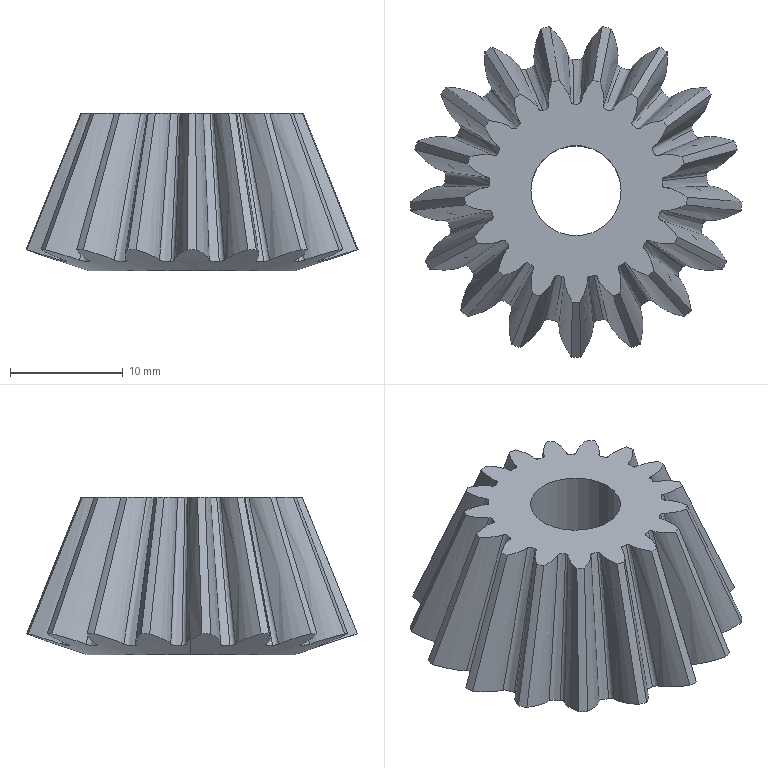Part | SolidWorks | features RefAxis 2, BlendCut 1, CirPattern 1, Revolution 1 | 1 solid | 91 faces | box 29.446 x 29.325 x 13.992 mm | volume 4731 mm3 | spline 68 | cone 19 | cylinder 2 | plane 2 | commonest cylinder face diameters 8 x2